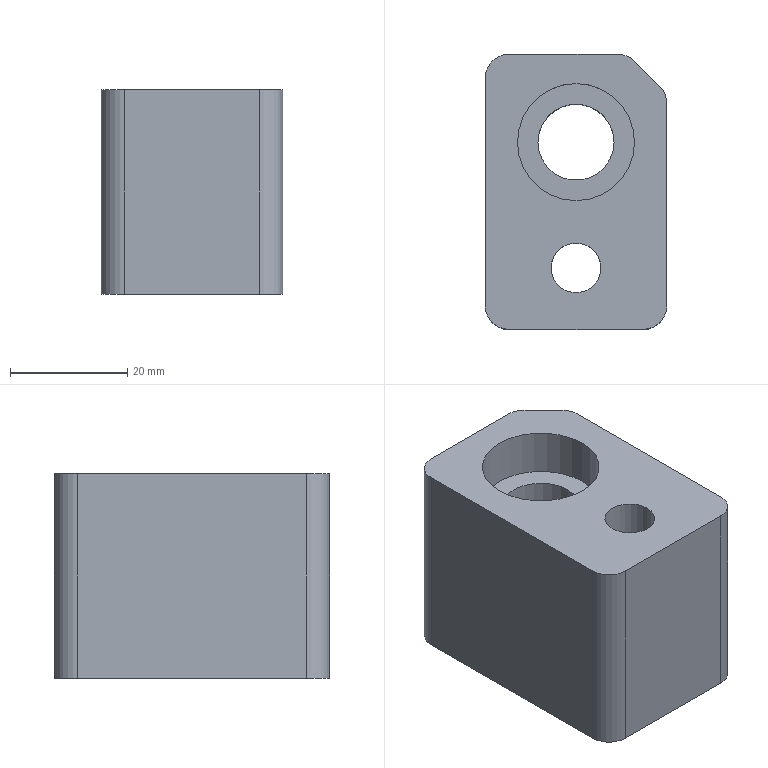Part | NX | features 7 2 | 1 solid | 18 faces | box 31 x 47 x 35 mm | volume 40131 mm3 | plane 9 | cylinder 9 | commonest cylinder face diameters 8 x5 8.5 x1 13 x1 14.5 x1 20 x1
STEP:
#1=CARTESIAN_POINT('',(97.029,411.95,91.));
#2=VERTEX_POINT('',#1);
#3=CARTESIAN_POINT('',(87.029,411.95,91.));
#4=DIRECTION('',(0.,0.,1.));
#5=DIRECTION('',(1.,0.,0.));
#6=AXIS2_PLACEMENT_3D('',#3,#4,#5);
#7=CIRCLE('',#6,10.);
#8=EDGE_CURVE('',#2,#2,#7,.T.);
#9=ORIENTED_EDGE('',*,*,#8,.F.);
#10=EDGE_LOOP('',(#9));
#11=FACE_BOUND('',#10,.T.);
#12=CARTESIAN_POINT('',(71.529,383.95,91.));
#13=VERTEX_POINT('',#12);
#14=CARTESIAN_POINT('',(71.529,422.95,91.));
#15=VERTEX_POINT('',#14);
#16=CARTESIAN_POINT('',(71.529,411.95,91.));
#17=DIRECTION('',(0.,1.,0.));
#18=VECTOR('',#17,1000.);
#19=LINE('',#16,#18);
#20=EDGE_CURVE('',#13,#15,#19,.T.);
#21=ORIENTED_EDGE('',*,*,#20,.F.);
#22=CARTESIAN_POINT('',(75.529,379.95,91.));
#23=VERTEX_POINT('',#22);
#24=CARTESIAN_POINT('',(75.529,383.95,91.));
#25=DIRECTION('',(0.,0.,1.));
#26=DIRECTION('',(1.,0.,0.));
#27=AXIS2_PLACEMENT_3D('',#24,#25,#26);
#28=CIRCLE('',#27,4.);
#29=EDGE_CURVE('',#13,#23,#28,.T.);
#30=ORIENTED_EDGE('',*,*,#29,.T.);
#31=CARTESIAN_POINT('',(98.529,379.95,91.));
#32=VERTEX_POINT('',#31);
#33=CARTESIAN_POINT('',(87.029,379.95,91.));
#34=DIRECTION('',(-1.,0.,0.));
#35=VECTOR('',#34,1000.);
#36=LINE('',#33,#35);
#37=EDGE_CURVE('',#32,#23,#36,.T.);
#38=ORIENTED_EDGE('',*,*,#37,.F.);
#39=CARTESIAN_POINT('',(102.529,383.95,91.));
#40=VERTEX_POINT('',#39);
#41=CARTESIAN_POINT('',(98.529,383.95,91.));
#42=DIRECTION('',(0.,0.,1.));
#43=DIRECTION('',(1.,0.,0.));
#44=AXIS2_PLACEMENT_3D('',#41,#42,#43);
#45=CIRCLE('',#44,4.);
#46=EDGE_CURVE('',#32,#40,#45,.T.);
#47=ORIENTED_EDGE('',*,*,#46,.T.);
#48=CARTESIAN_POINT('',(102.529,418.657,91.));
#49=VERTEX_POINT('',#48);
#50=CARTESIAN_POINT('',(102.529,411.95,91.));
#51=DIRECTION('',(0.,-1.,0.));
#52=VECTOR('',#51,1000.);
#53=LINE('',#50,#52);
#54=EDGE_CURVE('',#49,#40,#53,.T.);
#55=ORIENTED_EDGE('',*,*,#54,.F.);
#56=CARTESIAN_POINT('',(101.357,421.486,91.));
#57=VERTEX_POINT('',#56);
#58=CARTESIAN_POINT('',(98.529,418.657,91.));
#59=DIRECTION('',(0.,0.,1.));
#60=DIRECTION('',(1.,0.,0.));
#61=AXIS2_PLACEMENT_3D('',#58,#59,#60);
#62=CIRCLE('',#61,4.);
#63=EDGE_CURVE('',#49,#57,#62,.T.);
#64=ORIENTED_EDGE('',*,*,#63,.T.);
#65=CARTESIAN_POINT('',(97.064,425.778,91.));
#66=VERTEX_POINT('',#65);
#67=CARTESIAN_POINT('',(100.461,422.382,91.));
#68=DIRECTION('',(-0.7071,0.7071,0.));
#69=VECTOR('',#68,1000.);
#70=LINE('',#67,#69);
#71=EDGE_CURVE('',#57,#66,#70,.T.);
#72=ORIENTED_EDGE('',*,*,#71,.T.);
#73=CARTESIAN_POINT('',(94.236,426.95,91.));
#74=VERTEX_POINT('',#73);
#75=CARTESIAN_POINT('',(94.236,422.95,91.));
#76=DIRECTION('',(0.,0.,1.));
#77=DIRECTION('',(1.,0.,0.));
#78=AXIS2_PLACEMENT_3D('',#75,#76,#77);
#79=CIRCLE('',#78,4.);
#80=EDGE_CURVE('',#66,#74,#79,.T.);
#81=ORIENTED_EDGE('',*,*,#80,.T.);
#82=CARTESIAN_POINT('',(75.529,426.95,91.));
#83=VERTEX_POINT('',#82);
#84=CARTESIAN_POINT('',(87.029,426.95,91.));
#85=DIRECTION('',(1.,0.,0.));
#86=VECTOR('',#85,1000.);
#87=LINE('',#84,#86);
#88=EDGE_CURVE('',#83,#74,#87,.T.);
#89=ORIENTED_EDGE('',*,*,#88,.F.);
#90=CARTESIAN_POINT('',(75.529,422.95,91.));
#91=DIRECTION('',(0.,0.,1.));
#92=DIRECTION('',(1.,0.,0.));
#93=AXIS2_PLACEMENT_3D('',#90,#91,#92);
#94=CIRCLE('',#93,4.);
#95=EDGE_CURVE('',#83,#15,#94,.T.);
#96=ORIENTED_EDGE('',*,*,#95,.T.);
#97=EDGE_LOOP('',(#21,#30,#38,#47,#55,#64,#72,#81,#89,#96));
#98=FACE_BOUND('',#97,.T.);
#99=CARTESIAN_POINT('',(91.279,390.45,91.));
#100=VERTEX_POINT('',#99);
#101=CARTESIAN_POINT('',(87.029,390.45,91.));
#102=DIRECTION('',(0.,0.,-1.));
#103=DIRECTION('',(1.,0.,0.));
#104=AXIS2_PLACEMENT_3D('',#101,#102,#103);
#105=CIRCLE('',#104,4.25);
#106=EDGE_CURVE('',#100,#100,#105,.T.);
#107=ORIENTED_EDGE('',*,*,#106,.T.);
#108=EDGE_LOOP('',(#107));
#109=FACE_BOUND('',#108,.T.);
#110=CARTESIAN_POINT('',(87.029,409.45,91.));
#111=DIRECTION('',(0.,0.,1.));
#112=DIRECTION('',(-1.,0.,0.));
#113=AXIS2_PLACEMENT_3D('',#110,#111,#112);
#114=PLANE('',#113);
#115=ADVANCED_FACE('',(#11,#98,#109),#114,.T.);
#116=CARTESIAN_POINT('',(80.529,411.95,56.));
#117=VERTEX_POINT('',#116);
#118=CARTESIAN_POINT('',(87.029,411.95,56.));
#119=DIRECTION('',(0.,0.,-1.));
#120=DIRECTION('',(-1.,0.,0.));
#121=AXIS2_PLACEMENT_3D('',#118,#119,#120);
#122=CIRCLE('',#121,6.5);
#123=EDGE_CURVE('',#117,#117,#122,.T.);
#124=ORIENTED_EDGE('',*,*,#123,.F.);
#125=EDGE_LOOP('',(#124));
#126=FACE_BOUND('',#125,.T.);
#127=CARTESIAN_POINT('',(79.779,390.45,56.));
#128=VERTEX_POINT('',#127);
#129=CARTESIAN_POINT('',(87.029,390.45,56.));
#130=DIRECTION('',(0.,0.,-1.));
#131=DIRECTION('',(-1.,0.,0.));
#132=AXIS2_PLACEMENT_3D('',#129,#130,#131);
#133=CIRCLE('',#132,7.25);
#134=EDGE_CURVE('',#128,#128,#133,.T.);
#135=ORIENTED_EDGE('',*,*,#134,.F.);
#136=EDGE_LOOP('',(#135));
#137=FACE_BOUND('',#136,.T.);
#138=CARTESIAN_POINT('',(75.529,379.95,56.));
#139=VERTEX_POINT('',#138);
#140=CARTESIAN_POINT('',(98.529,379.95,56.));
#141=VERTEX_POINT('',#140);
#142=CARTESIAN_POINT('',(87.029,379.95,56.));
#143=DIRECTION('',(1.,0.,0.));
#144=VECTOR('',#143,1000.);
#145=LINE('',#142,#144);
#146=EDGE_CURVE('',#139,#141,#145,.T.);
#147=ORIENTED_EDGE('',*,*,#146,.F.);
#148=CARTESIAN_POINT('',(71.529,383.95,56.));
#149=VERTEX_POINT('',#148);
#150=CARTESIAN_POINT('',(75.529,383.95,56.));
#151=DIRECTION('',(0.,0.,-1.));
#152=DIRECTION('',(-1.,0.,0.));
#153=AXIS2_PLACEMENT_3D('',#150,#151,#152);
#154=CIRCLE('',#153,4.);
#155=EDGE_CURVE('',#139,#149,#154,.T.);
#156=ORIENTED_EDGE('',*,*,#155,.T.);
#157=CARTESIAN_POINT('',(71.529,422.95,56.));
#158=VERTEX_POINT('',#157);
#159=CARTESIAN_POINT('',(71.529,411.95,56.));
#160=DIRECTION('',(0.,-1.,0.));
#161=VECTOR('',#160,1000.);
#162=LINE('',#159,#161);
#163=EDGE_CURVE('',#158,#149,#162,.T.);
#164=ORIENTED_EDGE('',*,*,#163,.F.);
#165=CARTESIAN_POINT('',(75.529,426.95,56.));
#166=VERTEX_POINT('',#165);
#167=CARTESIAN_POINT('',(75.529,422.95,56.));
#168=DIRECTION('',(0.,0.,-1.));
#169=DIRECTION('',(-1.,0.,0.));
#170=AXIS2_PLACEMENT_3D('',#167,#168,#169);
#171=CIRCLE('',#170,4.);
#172=EDGE_CURVE('',#158,#166,#171,.T.);
#173=ORIENTED_EDGE('',*,*,#172,.T.);
#174=CARTESIAN_POINT('',(94.236,426.95,56.));
#175=VERTEX_POINT('',#174);
#176=CARTESIAN_POINT('',(87.029,426.95,56.));
#177=DIRECTION('',(-1.,0.,0.));
#178=VECTOR('',#177,1000.);
#179=LINE('',#176,#178);
#180=EDGE_CURVE('',#175,#166,#179,.T.);
#181=ORIENTED_EDGE('',*,*,#180,.F.);
#182=CARTESIAN_POINT('',(97.064,425.778,56.));
#183=VERTEX_POINT('',#182);
#184=CARTESIAN_POINT('',(94.236,422.95,56.));
#185=DIRECTION('',(0.,0.,-1.));
#186=DIRECTION('',(-1.,0.,0.));
#187=AXIS2_PLACEMENT_3D('',#184,#185,#186);
#188=CIRCLE('',#187,4.);
#189=EDGE_CURVE('',#175,#183,#188,.T.);
#190=ORIENTED_EDGE('',*,*,#189,.T.);
#191=CARTESIAN_POINT('',(101.357,421.486,56.));
#192=VERTEX_POINT('',#191);
#193=CARTESIAN_POINT('',(103.211,419.632,56.));
#194=DIRECTION('',(0.7071,-0.7071,0.));
#195=VECTOR('',#194,1000.);
#196=LINE('',#193,#195);
#197=EDGE_CURVE('',#183,#192,#196,.T.);
#198=ORIENTED_EDGE('',*,*,#197,.T.);
#199=CARTESIAN_POINT('',(102.529,418.657,56.));
#200=VERTEX_POINT('',#199);
#201=CARTESIAN_POINT('',(98.529,418.657,56.));
#202=DIRECTION('',(0.,0.,-1.));
#203=DIRECTION('',(-1.,0.,0.));
#204=AXIS2_PLACEMENT_3D('',#201,#202,#203);
#205=CIRCLE('',#204,4.);
#206=EDGE_CURVE('',#192,#200,#205,.T.);
#207=ORIENTED_EDGE('',*,*,#206,.T.);
#208=CARTESIAN_POINT('',(102.529,383.95,56.));
#209=VERTEX_POINT('',#208);
#210=CARTESIAN_POINT('',(102.529,411.95,56.));
#211=DIRECTION('',(0.,1.,0.));
#212=VECTOR('',#211,1000.);
#213=LINE('',#210,#212);
#214=EDGE_CURVE('',#209,#200,#213,.T.);
#215=ORIENTED_EDGE('',*,*,#214,.F.);
#216=CARTESIAN_POINT('',(98.529,383.95,56.));
#217=DIRECTION('',(0.,0.,-1.));
#218=DIRECTION('',(-1.,0.,0.));
#219=AXIS2_PLACEMENT_3D('',#216,#217,#218);
#220=CIRCLE('',#219,4.);
#221=EDGE_CURVE('',#209,#141,#220,.T.);
#222=ORIENTED_EDGE('',*,*,#221,.T.);
#223=EDGE_LOOP('',(#147,#156,#164,#173,#181,#190,#198,#207,#215,#222));
#224=FACE_BOUND('',#223,.T.);
#225=CARTESIAN_POINT('',(-89.971,226.95,56.));
#226=DIRECTION('',(0.,0.,-1.));
#227=DIRECTION('',(1.,0.,0.));
#228=AXIS2_PLACEMENT_3D('',#225,#226,#227);
#229=PLANE('',#228);
#230=ADVANCED_FACE('',(#126,#137,#224),#229,.T.);
#231=ORIENTED_EDGE('',*,*,#88,.T.);
#232=CARTESIAN_POINT('',(94.236,426.95,-5.));
#233=DIRECTION('',(0.,0.,-1.));
#234=VECTOR('',#233,1000.);
#235=LINE('',#232,#234);
#236=EDGE_CURVE('',#74,#175,#235,.T.);
#237=ORIENTED_EDGE('',*,*,#236,.T.);
#238=ORIENTED_EDGE('',*,*,#180,.T.);
#239=CARTESIAN_POINT('',(75.529,426.95,-5.));
#240=DIRECTION('',(0.,0.,1.));
#241=VECTOR('',#240,1000.);
#242=LINE('',#239,#241);
#243=EDGE_CURVE('',#166,#83,#242,.T.);
#244=ORIENTED_EDGE('',*,*,#243,.T.);
#245=EDGE_LOOP('',(#231,#237,#238,#244));
#246=FACE_BOUND('',#245,.T.);
#247=CARTESIAN_POINT('',(87.029,426.95,-5.));
#248=DIRECTION('',(0.,1.,0.));
#249=DIRECTION('',(0.,0.,-1.));
#250=AXIS2_PLACEMENT_3D('',#247,#248,#249);
#251=PLANE('',#250);
#252=ADVANCED_FACE('',(#246),#251,.T.);
#253=ORIENTED_EDGE('',*,*,#54,.T.);
#254=CARTESIAN_POINT('',(102.529,383.95,-5.));
#255=DIRECTION('',(0.,0.,-1.));
#256=VECTOR('',#255,1000.);
#257=LINE('',#254,#256);
#258=EDGE_CURVE('',#40,#209,#257,.T.);
#259=ORIENTED_EDGE('',*,*,#258,.T.);
#260=ORIENTED_EDGE('',*,*,#214,.T.);
#261=CARTESIAN_POINT('',(102.529,418.657,-5.));
#262=DIRECTION('',(0.,0.,1.));
#263=VECTOR('',#262,1000.);
#264=LINE('',#261,#263);
#265=EDGE_CURVE('',#200,#49,#264,.T.);
#266=ORIENTED_EDGE('',*,*,#265,.T.);
#267=EDGE_LOOP('',(#253,#259,#260,#266));
#268=FACE_BOUND('',#267,.T.);
#269=CARTESIAN_POINT('',(102.529,411.95,-5.));
#270=DIRECTION('',(1.,0.,0.));
#271=DIRECTION('',(0.,0.,1.));
#272=AXIS2_PLACEMENT_3D('',#269,#270,#271);
#273=PLANE('',#272);
#274=ADVANCED_FACE('',(#268),#273,.T.);
#275=ORIENTED_EDGE('',*,*,#37,.T.);
#276=CARTESIAN_POINT('',(75.529,379.95,-5.));
#277=DIRECTION('',(0.,0.,-1.));
#278=VECTOR('',#277,1000.);
#279=LINE('',#276,#278);
#280=EDGE_CURVE('',#23,#139,#279,.T.);
#281=ORIENTED_EDGE('',*,*,#280,.T.);
#282=ORIENTED_EDGE('',*,*,#146,.T.);
#283=CARTESIAN_POINT('',(98.529,379.95,-5.));
#284=DIRECTION('',(0.,0.,1.));
#285=VECTOR('',#284,1000.);
#286=LINE('',#283,#285);
#287=EDGE_CURVE('',#141,#32,#286,.T.);
#288=ORIENTED_EDGE('',*,*,#287,.T.);
#289=EDGE_LOOP('',(#275,#281,#282,#288));
#290=FACE_BOUND('',#289,.T.);
#291=CARTESIAN_POINT('',(87.029,379.95,-5.));
#292=DIRECTION('',(0.,-1.,0.));
#293=DIRECTION('',(0.,0.,1.));
#294=AXIS2_PLACEMENT_3D('',#291,#292,#293);
#295=PLANE('',#294);
#296=ADVANCED_FACE('',(#290),#295,.T.);
#297=ORIENTED_EDGE('',*,*,#163,.T.);
#298=CARTESIAN_POINT('',(71.529,383.95,-5.));
#299=DIRECTION('',(0.,0.,1.));
#300=VECTOR('',#299,1000.);
#301=LINE('',#298,#300);
#302=EDGE_CURVE('',#149,#13,#301,.T.);
#303=ORIENTED_EDGE('',*,*,#302,.T.);
#304=ORIENTED_EDGE('',*,*,#20,.T.);
#305=CARTESIAN_POINT('',(71.529,422.95,-5.));
#306=DIRECTION('',(0.,0.,-1.));
#307=VECTOR('',#306,1000.);
#308=LINE('',#305,#307);
#309=EDGE_CURVE('',#15,#158,#308,.T.);
#310=ORIENTED_EDGE('',*,*,#309,.T.);
#311=EDGE_LOOP('',(#297,#303,#304,#310));
#312=FACE_BOUND('',#311,.T.);
#313=CARTESIAN_POINT('',(71.529,411.95,-5.));
#314=DIRECTION('',(-1.,0.,0.));
#315=DIRECTION('',(0.,0.,-1.));
#316=AXIS2_PLACEMENT_3D('',#313,#314,#315);
#317=PLANE('',#316);
#318=ADVANCED_FACE('',(#312),#317,.T.);
#319=ORIENTED_EDGE('',*,*,#71,.F.);
#320=CARTESIAN_POINT('',(101.357,421.486,-5.));
#321=DIRECTION('',(0.,0.,-1.));
#322=VECTOR('',#321,1000.);
#323=LINE('',#320,#322);
#324=EDGE_CURVE('',#57,#192,#323,.T.);
#325=ORIENTED_EDGE('',*,*,#324,.T.);
#326=ORIENTED_EDGE('',*,*,#197,.F.);
#327=CARTESIAN_POINT('',(97.064,425.778,-5.));
#328=DIRECTION('',(0.,0.,1.));
#329=VECTOR('',#328,1000.);
#330=LINE('',#327,#329);
#331=EDGE_CURVE('',#183,#66,#330,.T.);
#332=ORIENTED_EDGE('',*,*,#331,.T.);
#333=EDGE_LOOP('',(#319,#325,#326,#332));
#334=FACE_BOUND('',#333,.T.);
#335=CARTESIAN_POINT('',(103.211,419.632,-5.));
#336=DIRECTION('',(-0.7071,-0.7071,0.));
#337=DIRECTION('',(0.,0.,1.));
#338=AXIS2_PLACEMENT_3D('',#335,#336,#337);
#339=PLANE('',#338);
#340=ADVANCED_FACE('',(#334),#339,.F.);
#341=ORIENTED_EDGE('',*,*,#155,.F.);
#342=ORIENTED_EDGE('',*,*,#280,.F.);
#343=ORIENTED_EDGE('',*,*,#29,.F.);
#344=ORIENTED_EDGE('',*,*,#302,.F.);
#345=EDGE_LOOP('',(#341,#342,#343,#344));
#346=FACE_BOUND('',#345,.T.);
#347=CARTESIAN_POINT('',(75.529,383.95,-5.));
#348=DIRECTION('',(0.,0.,-1.));
#349=DIRECTION('',(-1.,0.,0.));
#350=AXIS2_PLACEMENT_3D('',#347,#348,#349);
#351=CYLINDRICAL_SURFACE('',#350,4.);
#352=ADVANCED_FACE('',(#346),#351,.T.);
#353=ORIENTED_EDGE('',*,*,#221,.F.);
#354=ORIENTED_EDGE('',*,*,#258,.F.);
#355=ORIENTED_EDGE('',*,*,#46,.F.);
#356=ORIENTED_EDGE('',*,*,#287,.F.);
#357=EDGE_LOOP('',(#353,#354,#355,#356));
#358=FACE_BOUND('',#357,.T.);
#359=CARTESIAN_POINT('',(98.529,383.95,-5.));
#360=DIRECTION('',(0.,0.,-1.));
#361=DIRECTION('',(-1.,0.,0.));
#362=AXIS2_PLACEMENT_3D('',#359,#360,#361);
#363=CYLINDRICAL_SURFACE('',#362,4.);
#364=ADVANCED_FACE('',(#358),#363,.T.);
#365=ORIENTED_EDGE('',*,*,#206,.F.);
#366=ORIENTED_EDGE('',*,*,#324,.F.);
#367=ORIENTED_EDGE('',*,*,#63,.F.);
#368=ORIENTED_EDGE('',*,*,#265,.F.);
#369=EDGE_LOOP('',(#365,#366,#367,#368));
#370=FACE_BOUND('',#369,.T.);
#371=CARTESIAN_POINT('',(98.529,418.657,-5.));
#372=DIRECTION('',(0.,0.,1.));
#373=DIRECTION('',(1.,0.,0.));
#374=AXIS2_PLACEMENT_3D('',#371,#372,#373);
#375=CYLINDRICAL_SURFACE('',#374,4.);
#376=ADVANCED_FACE('',(#370),#375,.T.);
#377=ORIENTED_EDGE('',*,*,#80,.F.);
#378=ORIENTED_EDGE('',*,*,#331,.F.);
#379=ORIENTED_EDGE('',*,*,#189,.F.);
#380=ORIENTED_EDGE('',*,*,#236,.F.);
#381=EDGE_LOOP('',(#377,#378,#379,#380));
#382=FACE_BOUND('',#381,.T.);
#383=CARTESIAN_POINT('',(94.236,422.95,-5.));
#384=DIRECTION('',(0.,0.,-1.));
#385=DIRECTION('',(-1.,0.,0.));
#386=AXIS2_PLACEMENT_3D('',#383,#384,#385);
#387=CYLINDRICAL_SURFACE('',#386,4.);
#388=ADVANCED_FACE('',(#382),#387,.T.);
#389=ORIENTED_EDGE('',*,*,#172,.F.);
#390=ORIENTED_EDGE('',*,*,#309,.F.);
#391=ORIENTED_EDGE('',*,*,#95,.F.);
#392=ORIENTED_EDGE('',*,*,#243,.F.);
#393=EDGE_LOOP('',(#389,#390,#391,#392));
#394=FACE_BOUND('',#393,.T.);
#395=CARTESIAN_POINT('',(75.529,422.95,-5.));
#396=DIRECTION('',(0.,0.,-1.));
#397=DIRECTION('',(-1.,0.,0.));
#398=AXIS2_PLACEMENT_3D('',#395,#396,#397);
#399=CYLINDRICAL_SURFACE('',#398,4.);
#400=ADVANCED_FACE('',(#394),#399,.T.);
#401=CARTESIAN_POINT('',(91.279,390.45,71.));
#402=VERTEX_POINT('',#401);
#403=CARTESIAN_POINT('',(87.029,390.45,71.));
#404=DIRECTION('',(0.,0.,1.));
#405=DIRECTION('',(1.,0.,0.));
#406=AXIS2_PLACEMENT_3D('',#403,#404,#405);
#407=CIRCLE('',#406,4.25);
#408=EDGE_CURVE('',#402,#402,#407,.T.);
#409=ORIENTED_EDGE('',*,*,#408,.F.);
#410=EDGE_LOOP('',(#409));
#411=FACE_BOUND('',#410,.T.);
#412=ORIENTED_EDGE('',*,*,#106,.F.);
#413=EDGE_LOOP('',(#412));
#414=FACE_BOUND('',#413,.T.);
#415=CARTESIAN_POINT('',(87.029,390.45,55.));
#416=DIRECTION('',(0.,0.,1.));
#417=DIRECTION('',(-1.,0.,0.));
#418=AXIS2_PLACEMENT_3D('',#415,#416,#417);
#419=CYLINDRICAL_SURFACE('',#418,4.25);
#420=ADVANCED_FACE('',(#411,#414),#419,.F.);
#421=ORIENTED_EDGE('',*,*,#408,.T.);
#422=EDGE_LOOP('',(#421));
#423=FACE_BOUND('',#422,.T.);
#424=CARTESIAN_POINT('',(94.279,390.45,71.));
#425=VERTEX_POINT('',#424);
#426=CARTESIAN_POINT('',(87.029,390.45,71.));
#427=DIRECTION('',(0.,0.,1.));
#428=DIRECTION('',(1.,0.,0.));
#429=AXIS2_PLACEMENT_3D('',#426,#427,#428);
#430=CIRCLE('',#429,7.25);
#431=EDGE_CURVE('',#425,#425,#430,.T.);
#432=ORIENTED_EDGE('',*,*,#431,.F.);
#433=EDGE_LOOP('',(#432));
#434=FACE_BOUND('',#433,.T.);
#435=CARTESIAN_POINT('',(87.029,390.45,71.));
#436=DIRECTION('',(0.,0.,1.));
#437=DIRECTION('',(-1.,0.,0.));
#438=AXIS2_PLACEMENT_3D('',#435,#436,#437);
#439=PLANE('',#438);
#440=ADVANCED_FACE('',(#423,#434),#439,.F.);
#441=ORIENTED_EDGE('',*,*,#134,.T.);
#442=EDGE_LOOP('',(#441));
#443=FACE_BOUND('',#442,.T.);
#444=ORIENTED_EDGE('',*,*,#431,.T.);
#445=EDGE_LOOP('',(#444));
#446=FACE_BOUND('',#445,.T.);
#447=CARTESIAN_POINT('',(87.029,390.45,55.));
#448=DIRECTION('',(0.,0.,1.));
#449=DIRECTION('',(-1.,0.,0.));
#450=AXIS2_PLACEMENT_3D('',#447,#448,#449);
#451=CYLINDRICAL_SURFACE('',#450,7.25);
#452=ADVANCED_FACE('',(#443,#446),#451,.F.);
#453=CARTESIAN_POINT('',(80.529,411.95,83.));
#454=VERTEX_POINT('',#453);
#455=CARTESIAN_POINT('',(87.029,411.95,83.));
#456=DIRECTION('',(0.,0.,1.));
#457=DIRECTION('',(-1.,0.,0.));
#458=AXIS2_PLACEMENT_3D('',#455,#456,#457);
#459=CIRCLE('',#458,6.5);
#460=EDGE_CURVE('',#454,#454,#459,.T.);
#461=ORIENTED_EDGE('',*,*,#460,.T.);
#462=EDGE_LOOP('',(#461));
#463=FACE_BOUND('',#462,.T.);
#464=ORIENTED_EDGE('',*,*,#123,.T.);
#465=EDGE_LOOP('',(#464));
#466=FACE_BOUND('',#465,.T.);
#467=CARTESIAN_POINT('',(87.029,411.95,91.));
#468=DIRECTION('',(0.,0.,-1.));
#469=DIRECTION('',(-1.,0.,0.));
#470=AXIS2_PLACEMENT_3D('',#467,#468,#469);
#471=CYLINDRICAL_SURFACE('',#470,6.5);
#472=ADVANCED_FACE('',(#463,#466),#471,.F.);
#473=CARTESIAN_POINT('',(77.029,411.95,83.));
#474=VERTEX_POINT('',#473);
#475=CARTESIAN_POINT('',(87.029,411.95,83.));
#476=DIRECTION('',(0.,0.,-1.));
#477=DIRECTION('',(-1.,0.,0.));
#478=AXIS2_PLACEMENT_3D('',#475,#476,#477);
#479=CIRCLE('',#478,10.);
#480=EDGE_CURVE('',#474,#474,#479,.T.);
#481=ORIENTED_EDGE('',*,*,#480,.F.);
#482=EDGE_LOOP('',(#481));
#483=FACE_BOUND('',#482,.T.);
#484=ORIENTED_EDGE('',*,*,#460,.F.);
#485=EDGE_LOOP('',(#484));
#486=FACE_BOUND('',#485,.T.);
#487=CARTESIAN_POINT('',(87.029,411.95,83.));
#488=DIRECTION('',(0.,0.,-1.));
#489=DIRECTION('',(-1.,0.,0.));
#490=AXIS2_PLACEMENT_3D('',#487,#488,#489);
#491=PLANE('',#490);
#492=ADVANCED_FACE('',(#483,#486),#491,.F.);
#493=ORIENTED_EDGE('',*,*,#8,.T.);
#494=EDGE_LOOP('',(#493));
#495=FACE_BOUND('',#494,.T.);
#496=ORIENTED_EDGE('',*,*,#480,.T.);
#497=EDGE_LOOP('',(#496));
#498=FACE_BOUND('',#497,.T.);
#499=CARTESIAN_POINT('',(87.029,411.95,90.559));
#500=DIRECTION('',(0.,0.,-1.));
#501=DIRECTION('',(1.,0.,0.));
#502=AXIS2_PLACEMENT_3D('',#499,#500,#501);
#503=CYLINDRICAL_SURFACE('',#502,10.);
#504=ADVANCED_FACE('',(#495,#498),#503,.F.);
#505=CLOSED_SHELL('',(#115,#230,#252,#274,#296,#318,#340,#352,#364,#376,#388,#400,#420,#440,#452,#472,#492,#504));
#506=MANIFOLD_SOLID_BREP('',#505);
#507=(LENGTH_UNIT()NAMED_UNIT(*)SI_UNIT(.MILLI.,.METRE.));
#508=UNCERTAINTY_MEASURE_WITH_UNIT(LENGTH_MEASURE(0.00001),#507,'','');
#509=(NAMED_UNIT(*)PLANE_ANGLE_UNIT()SI_UNIT($,.RADIAN.));
#510=(NAMED_UNIT(*)SI_UNIT($,.STERADIAN.)SOLID_ANGLE_UNIT());
#511=(GEOMETRIC_REPRESENTATION_CONTEXT(3)GLOBAL_UNCERTAINTY_ASSIGNED_CONTEXT((#508))GLOBAL_UNIT_ASSIGNED_CONTEXT((#507,#509,#510))REPRESENTATION_CONTEXT('',''));
#512=ADVANCED_BREP_SHAPE_REPRESENTATION('',(#506),#511);